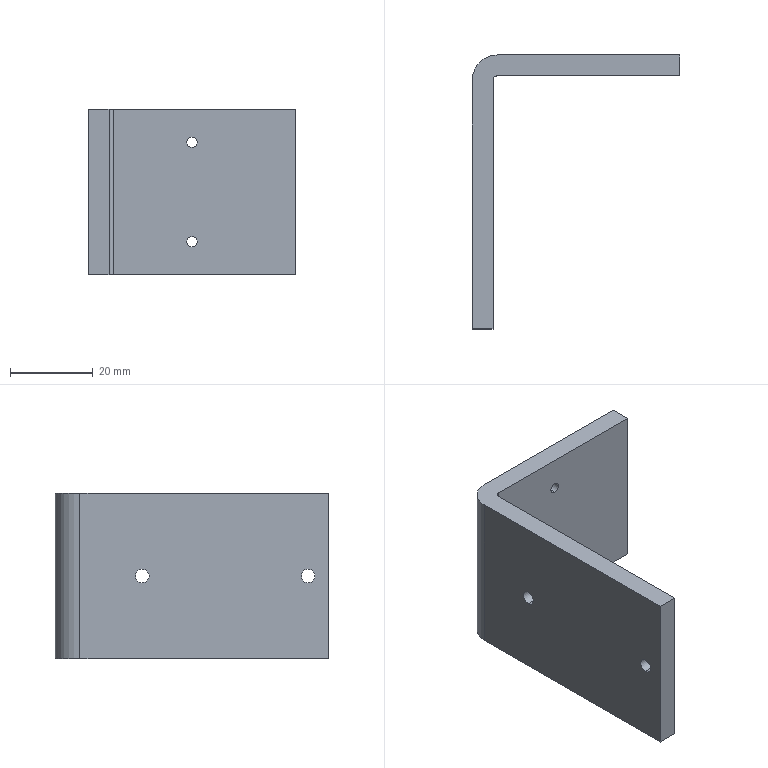Part | STEP file | X77-04302 | 1 solid | 18 faces | box 50 x 66 x 40 mm | volume 21765 mm3 | cylinder 10 | plane 8 | commonest cylinder face diameters 2.5 x4 3.3 x4 2 x1 12 x1
STEP:
#1=CARTESIAN_POINT('',(-24.91,-36.8,13.25));
#2=VERTEX_POINT('',#1);
#3=CARTESIAN_POINT('',(-24.91,-36.8,10.75));
#4=VERTEX_POINT('',#3);
#5=CARTESIAN_POINT('',(-24.91,-36.8,12.));
#6=DIRECTION('',(0.,-1.,0.));
#7=DIRECTION('',(1.,0.,0.));
#8=AXIS2_PLACEMENT_3D('',#5,#6,#7);
#9=CIRCLE('',#8,1.25);
#10=EDGE_CURVE('',#2,#4,#9,.T.);
#11=ORIENTED_EDGE('',*,*,#10,.T.);
#12=CARTESIAN_POINT('',(-24.91,-31.8,10.75));
#13=VERTEX_POINT('',#12);
#14=CARTESIAN_POINT('',(-24.91,-31.8,10.75));
#15=DIRECTION('',(0.,1.,0.));
#16=VECTOR('',#15,1000.);
#17=LINE('',#14,#16);
#18=EDGE_CURVE('',#4,#13,#17,.T.);
#19=ORIENTED_EDGE('',*,*,#18,.T.);
#20=CARTESIAN_POINT('',(-24.91,-31.8,13.25));
#21=VERTEX_POINT('',#20);
#22=CARTESIAN_POINT('',(-24.91,-31.8,12.));
#23=DIRECTION('',(0.,1.,0.));
#24=DIRECTION('',(0.,0.,1.));
#25=AXIS2_PLACEMENT_3D('',#22,#23,#24);
#26=CIRCLE('',#25,1.25);
#27=EDGE_CURVE('',#13,#21,#26,.T.);
#28=ORIENTED_EDGE('',*,*,#27,.T.);
#29=CARTESIAN_POINT('',(-24.91,-31.8,13.25));
#30=DIRECTION('',(0.,1.,0.));
#31=VECTOR('',#30,1000.);
#32=LINE('',#29,#31);
#33=EDGE_CURVE('',#2,#21,#32,.T.);
#34=ORIENTED_EDGE('',*,*,#33,.F.);
#35=EDGE_LOOP('',(#11,#19,#28,#34));
#36=FACE_OUTER_BOUND('',#35,.T.);
#37=CARTESIAN_POINT('',(-24.91,-31.8,12.));
#38=DIRECTION('',(0.,1.,0.));
#39=DIRECTION('',(0.,0.,1.));
#40=AXIS2_PLACEMENT_3D('',#37,#38,#39);
#41=CYLINDRICAL_SURFACE('',#40,1.25);
#42=ADVANCED_FACE('',(#36),#41,.F.);
#43=CARTESIAN_POINT('',(-24.91,-36.8,-10.75));
#44=VERTEX_POINT('',#43);
#45=CARTESIAN_POINT('',(-24.91,-36.8,-13.25));
#46=VERTEX_POINT('',#45);
#47=CARTESIAN_POINT('',(-24.91,-36.8,-12.));
#48=DIRECTION('',(0.,-1.,0.));
#49=DIRECTION('',(1.,0.,0.));
#50=AXIS2_PLACEMENT_3D('',#47,#48,#49);
#51=CIRCLE('',#50,1.25);
#52=EDGE_CURVE('',#44,#46,#51,.T.);
#53=ORIENTED_EDGE('',*,*,#52,.T.);
#54=CARTESIAN_POINT('',(-24.91,-31.8,-13.25));
#55=VERTEX_POINT('',#54);
#56=CARTESIAN_POINT('',(-24.91,-31.8,-13.25));
#57=DIRECTION('',(0.,1.,0.));
#58=VECTOR('',#57,1000.);
#59=LINE('',#56,#58);
#60=EDGE_CURVE('',#46,#55,#59,.T.);
#61=ORIENTED_EDGE('',*,*,#60,.T.);
#62=CARTESIAN_POINT('',(-24.91,-31.8,-10.75));
#63=VERTEX_POINT('',#62);
#64=CARTESIAN_POINT('',(-24.91,-31.8,-12.));
#65=DIRECTION('',(0.,1.,0.));
#66=DIRECTION('',(0.,0.,1.));
#67=AXIS2_PLACEMENT_3D('',#64,#65,#66);
#68=CIRCLE('',#67,1.25);
#69=EDGE_CURVE('',#55,#63,#68,.T.);
#70=ORIENTED_EDGE('',*,*,#69,.T.);
#71=CARTESIAN_POINT('',(-24.91,-31.8,-10.75));
#72=DIRECTION('',(0.,1.,0.));
#73=VECTOR('',#72,1000.);
#74=LINE('',#71,#73);
#75=EDGE_CURVE('',#44,#63,#74,.T.);
#76=ORIENTED_EDGE('',*,*,#75,.F.);
#77=EDGE_LOOP('',(#53,#61,#70,#76));
#78=FACE_OUTER_BOUND('',#77,.T.);
#79=CARTESIAN_POINT('',(-24.91,-31.8,-12.));
#80=DIRECTION('',(0.,1.,0.));
#81=DIRECTION('',(0.,0.,1.));
#82=AXIS2_PLACEMENT_3D('',#79,#80,#81);
#83=CYLINDRICAL_SURFACE('',#82,1.25);
#84=ADVANCED_FACE('',(#78),#83,.F.);
#85=CARTESIAN_POINT('',(-44.91,-92.8,1.65));
#86=VERTEX_POINT('',#85);
#87=CARTESIAN_POINT('',(-44.91,-92.8,-1.65));
#88=VERTEX_POINT('',#87);
#89=CARTESIAN_POINT('',(-44.91,-92.8,0.));
#90=DIRECTION('',(1.,0.,0.));
#91=DIRECTION('',(0.,0.,-1.));
#92=AXIS2_PLACEMENT_3D('',#89,#90,#91);
#93=CIRCLE('',#92,1.65);
#94=EDGE_CURVE('',#86,#88,#93,.T.);
#95=ORIENTED_EDGE('',*,*,#94,.T.);
#96=CARTESIAN_POINT('',(-49.91,-92.8,-1.65));
#97=VERTEX_POINT('',#96);
#98=CARTESIAN_POINT('',(-49.91,-92.8,-1.65));
#99=DIRECTION('',(-1.,0.,0.));
#100=VECTOR('',#99,1000.);
#101=LINE('',#98,#100);
#102=EDGE_CURVE('',#88,#97,#101,.T.);
#103=ORIENTED_EDGE('',*,*,#102,.T.);
#104=CARTESIAN_POINT('',(-49.91,-92.8,1.65));
#105=VERTEX_POINT('',#104);
#106=CARTESIAN_POINT('',(-49.91,-92.8,0.));
#107=DIRECTION('',(-1.,0.,0.));
#108=DIRECTION('',(0.,0.,1.));
#109=AXIS2_PLACEMENT_3D('',#106,#107,#108);
#110=CIRCLE('',#109,1.65);
#111=EDGE_CURVE('',#97,#105,#110,.T.);
#112=ORIENTED_EDGE('',*,*,#111,.T.);
#113=CARTESIAN_POINT('',(-49.91,-92.8,1.65));
#114=DIRECTION('',(-1.,0.,0.));
#115=VECTOR('',#114,1000.);
#116=LINE('',#113,#115);
#117=EDGE_CURVE('',#86,#105,#116,.T.);
#118=ORIENTED_EDGE('',*,*,#117,.F.);
#119=EDGE_LOOP('',(#95,#103,#112,#118));
#120=FACE_OUTER_BOUND('',#119,.T.);
#121=CARTESIAN_POINT('',(-49.91,-92.8,0.));
#122=DIRECTION('',(-1.,0.,0.));
#123=DIRECTION('',(0.,0.,1.));
#124=AXIS2_PLACEMENT_3D('',#121,#122,#123);
#125=CYLINDRICAL_SURFACE('',#124,1.65);
#126=ADVANCED_FACE('',(#120),#125,.F.);
#127=CARTESIAN_POINT('',(-44.91,-52.8,1.65));
#128=VERTEX_POINT('',#127);
#129=CARTESIAN_POINT('',(-44.91,-52.8,-1.65));
#130=VERTEX_POINT('',#129);
#131=CARTESIAN_POINT('',(-44.91,-52.8,0.));
#132=DIRECTION('',(1.,0.,0.));
#133=DIRECTION('',(0.,0.,-1.));
#134=AXIS2_PLACEMENT_3D('',#131,#132,#133);
#135=CIRCLE('',#134,1.65);
#136=EDGE_CURVE('',#128,#130,#135,.T.);
#137=ORIENTED_EDGE('',*,*,#136,.T.);
#138=CARTESIAN_POINT('',(-49.91,-52.8,-1.65));
#139=VERTEX_POINT('',#138);
#140=CARTESIAN_POINT('',(-49.91,-52.8,-1.65));
#141=DIRECTION('',(-1.,0.,0.));
#142=VECTOR('',#141,1000.);
#143=LINE('',#140,#142);
#144=EDGE_CURVE('',#130,#139,#143,.T.);
#145=ORIENTED_EDGE('',*,*,#144,.T.);
#146=CARTESIAN_POINT('',(-49.91,-52.8,1.65));
#147=VERTEX_POINT('',#146);
#148=CARTESIAN_POINT('',(-49.91,-52.8,0.));
#149=DIRECTION('',(-1.,0.,0.));
#150=DIRECTION('',(0.,0.,1.));
#151=AXIS2_PLACEMENT_3D('',#148,#149,#150);
#152=CIRCLE('',#151,1.65);
#153=EDGE_CURVE('',#139,#147,#152,.T.);
#154=ORIENTED_EDGE('',*,*,#153,.T.);
#155=CARTESIAN_POINT('',(-49.91,-52.8,1.65));
#156=DIRECTION('',(-1.,0.,0.));
#157=VECTOR('',#156,1000.);
#158=LINE('',#155,#157);
#159=EDGE_CURVE('',#128,#147,#158,.T.);
#160=ORIENTED_EDGE('',*,*,#159,.F.);
#161=EDGE_LOOP('',(#137,#145,#154,#160));
#162=FACE_OUTER_BOUND('',#161,.T.);
#163=CARTESIAN_POINT('',(-49.91,-52.8,0.));
#164=DIRECTION('',(-1.,0.,0.));
#165=DIRECTION('',(0.,0.,1.));
#166=AXIS2_PLACEMENT_3D('',#163,#164,#165);
#167=CYLINDRICAL_SURFACE('',#166,1.65);
#168=ADVANCED_FACE('',(#162),#167,.F.);
#169=CARTESIAN_POINT('',(0.09,-31.8,-20.));
#170=VERTEX_POINT('',#169);
#171=CARTESIAN_POINT('',(0.09,-31.8,20.));
#172=VERTEX_POINT('',#171);
#173=CARTESIAN_POINT('',(0.09,-31.8,-20.));
#174=DIRECTION('',(0.,0.,1.));
#175=VECTOR('',#174,1000.);
#176=LINE('',#173,#175);
#177=EDGE_CURVE('',#170,#172,#176,.T.);
#178=ORIENTED_EDGE('',*,*,#177,.T.);
#179=CARTESIAN_POINT('',(0.09,-36.8,20.));
#180=VERTEX_POINT('',#179);
#181=CARTESIAN_POINT('',(0.09,-31.8,20.));
#182=DIRECTION('',(0.,1.,0.));
#183=VECTOR('',#182,1000.);
#184=LINE('',#181,#183);
#185=EDGE_CURVE('',#180,#172,#184,.T.);
#186=ORIENTED_EDGE('',*,*,#185,.F.);
#187=CARTESIAN_POINT('',(0.09,-36.8,-20.));
#188=VERTEX_POINT('',#187);
#189=CARTESIAN_POINT('',(0.09,-36.8,-20.));
#190=DIRECTION('',(0.,0.,1.));
#191=VECTOR('',#190,1000.);
#192=LINE('',#189,#191);
#193=EDGE_CURVE('',#188,#180,#192,.T.);
#194=ORIENTED_EDGE('',*,*,#193,.F.);
#195=CARTESIAN_POINT('',(0.09,-31.8,-20.));
#196=DIRECTION('',(0.,1.,0.));
#197=VECTOR('',#196,1000.);
#198=LINE('',#195,#197);
#199=EDGE_CURVE('',#188,#170,#198,.T.);
#200=ORIENTED_EDGE('',*,*,#199,.T.);
#201=EDGE_LOOP('',(#178,#186,#194,#200));
#202=FACE_OUTER_BOUND('',#201,.T.);
#203=CARTESIAN_POINT('',(0.09,-31.8,-20.));
#204=DIRECTION('',(1.,0.,0.));
#205=DIRECTION('',(0.,1.,0.));
#206=AXIS2_PLACEMENT_3D('',#203,#204,#205);
#207=PLANE('',#206);
#208=ADVANCED_FACE('',(#202),#207,.T.);
#209=ORIENTED_EDGE('',*,*,#10,.F.);
#210=CARTESIAN_POINT('',(-24.91,-36.8,12.));
#211=DIRECTION('',(0.,-1.,0.));
#212=DIRECTION('',(1.,0.,0.));
#213=AXIS2_PLACEMENT_3D('',#210,#211,#212);
#214=CIRCLE('',#213,1.25);
#215=EDGE_CURVE('',#4,#2,#214,.T.);
#216=ORIENTED_EDGE('',*,*,#215,.F.);
#217=EDGE_LOOP('',(#209,#216));
#218=FACE_BOUND('',#217,.T.);
#219=ORIENTED_EDGE('',*,*,#52,.F.);
#220=CARTESIAN_POINT('',(-24.91,-36.8,-12.));
#221=DIRECTION('',(0.,-1.,0.));
#222=DIRECTION('',(1.,0.,0.));
#223=AXIS2_PLACEMENT_3D('',#220,#221,#222);
#224=CIRCLE('',#223,1.25);
#225=EDGE_CURVE('',#46,#44,#224,.T.);
#226=ORIENTED_EDGE('',*,*,#225,.F.);
#227=EDGE_LOOP('',(#219,#226));
#228=FACE_BOUND('',#227,.T.);
#229=ORIENTED_EDGE('',*,*,#193,.T.);
#230=CARTESIAN_POINT('',(-43.91,-36.8,20.));
#231=VERTEX_POINT('',#230);
#232=CARTESIAN_POINT('',(0.09,-36.8,20.));
#233=DIRECTION('',(1.,0.,0.));
#234=VECTOR('',#233,1000.);
#235=LINE('',#232,#234);
#236=EDGE_CURVE('',#231,#180,#235,.T.);
#237=ORIENTED_EDGE('',*,*,#236,.F.);
#238=CARTESIAN_POINT('',(-43.91,-36.8,-20.));
#239=VERTEX_POINT('',#238);
#240=CARTESIAN_POINT('',(-43.91,-36.8,-20.));
#241=DIRECTION('',(0.,0.,1.));
#242=VECTOR('',#241,1000.);
#243=LINE('',#240,#242);
#244=EDGE_CURVE('',#239,#231,#243,.T.);
#245=ORIENTED_EDGE('',*,*,#244,.F.);
#246=CARTESIAN_POINT('',(0.09,-36.8,-20.));
#247=DIRECTION('',(1.,0.,0.));
#248=VECTOR('',#247,1000.);
#249=LINE('',#246,#248);
#250=EDGE_CURVE('',#239,#188,#249,.T.);
#251=ORIENTED_EDGE('',*,*,#250,.T.);
#252=EDGE_LOOP('',(#229,#237,#245,#251));
#253=FACE_OUTER_BOUND('',#252,.T.);
#254=CARTESIAN_POINT('',(0.09,-36.8,-20.));
#255=DIRECTION('',(0.,-1.,0.));
#256=DIRECTION('',(1.,0.,0.));
#257=AXIS2_PLACEMENT_3D('',#254,#255,#256);
#258=PLANE('',#257);
#259=ADVANCED_FACE('',(#218,#228,#253),#258,.T.);
#260=ORIENTED_EDGE('',*,*,#244,.T.);
#261=CARTESIAN_POINT('',(-44.91,-37.8,20.));
#262=VERTEX_POINT('',#261);
#263=CARTESIAN_POINT('',(-43.91,-37.8,20.));
#264=DIRECTION('',(0.,0.,-1.));
#265=DIRECTION('',(-1.,0.,0.));
#266=AXIS2_PLACEMENT_3D('',#263,#264,#265);
#267=CIRCLE('',#266,1.);
#268=EDGE_CURVE('',#262,#231,#267,.T.);
#269=ORIENTED_EDGE('',*,*,#268,.F.);
#270=CARTESIAN_POINT('',(-44.91,-37.8,-20.));
#271=VERTEX_POINT('',#270);
#272=CARTESIAN_POINT('',(-44.91,-37.8,-20.));
#273=DIRECTION('',(0.,0.,1.));
#274=VECTOR('',#273,1000.);
#275=LINE('',#272,#274);
#276=EDGE_CURVE('',#271,#262,#275,.T.);
#277=ORIENTED_EDGE('',*,*,#276,.F.);
#278=CARTESIAN_POINT('',(-43.91,-37.8,-20.));
#279=DIRECTION('',(0.,0.,-1.));
#280=DIRECTION('',(-1.,0.,0.));
#281=AXIS2_PLACEMENT_3D('',#278,#279,#280);
#282=CIRCLE('',#281,1.);
#283=EDGE_CURVE('',#271,#239,#282,.T.);
#284=ORIENTED_EDGE('',*,*,#283,.T.);
#285=EDGE_LOOP('',(#260,#269,#277,#284));
#286=FACE_OUTER_BOUND('',#285,.T.);
#287=CARTESIAN_POINT('',(-43.91,-37.8,-20.));
#288=DIRECTION('',(0.,0.,1.));
#289=DIRECTION('',(1.,0.,0.));
#290=AXIS2_PLACEMENT_3D('',#287,#288,#289);
#291=CYLINDRICAL_SURFACE('',#290,1.);
#292=ADVANCED_FACE('',(#286),#291,.F.);
#293=ORIENTED_EDGE('',*,*,#94,.F.);
#294=CARTESIAN_POINT('',(-44.91,-92.8,0.));
#295=DIRECTION('',(1.,0.,0.));
#296=DIRECTION('',(0.,0.,-1.));
#297=AXIS2_PLACEMENT_3D('',#294,#295,#296);
#298=CIRCLE('',#297,1.65);
#299=EDGE_CURVE('',#88,#86,#298,.T.);
#300=ORIENTED_EDGE('',*,*,#299,.F.);
#301=EDGE_LOOP('',(#293,#300));
#302=FACE_BOUND('',#301,.T.);
#303=ORIENTED_EDGE('',*,*,#136,.F.);
#304=CARTESIAN_POINT('',(-44.91,-52.8,0.));
#305=DIRECTION('',(1.,0.,0.));
#306=DIRECTION('',(0.,0.,-1.));
#307=AXIS2_PLACEMENT_3D('',#304,#305,#306);
#308=CIRCLE('',#307,1.65);
#309=EDGE_CURVE('',#130,#128,#308,.T.);
#310=ORIENTED_EDGE('',*,*,#309,.F.);
#311=EDGE_LOOP('',(#303,#310));
#312=FACE_BOUND('',#311,.T.);
#313=ORIENTED_EDGE('',*,*,#276,.T.);
#314=CARTESIAN_POINT('',(-44.91,-97.8,20.));
#315=VERTEX_POINT('',#314);
#316=CARTESIAN_POINT('',(-44.91,-37.8,20.));
#317=DIRECTION('',(0.,1.,0.));
#318=VECTOR('',#317,1000.);
#319=LINE('',#316,#318);
#320=EDGE_CURVE('',#315,#262,#319,.T.);
#321=ORIENTED_EDGE('',*,*,#320,.F.);
#322=CARTESIAN_POINT('',(-44.91,-97.8,-20.));
#323=VERTEX_POINT('',#322);
#324=CARTESIAN_POINT('',(-44.91,-97.8,-20.));
#325=DIRECTION('',(0.,0.,1.));
#326=VECTOR('',#325,1000.);
#327=LINE('',#324,#326);
#328=EDGE_CURVE('',#323,#315,#327,.T.);
#329=ORIENTED_EDGE('',*,*,#328,.F.);
#330=CARTESIAN_POINT('',(-44.91,-37.8,-20.));
#331=DIRECTION('',(0.,1.,0.));
#332=VECTOR('',#331,1000.);
#333=LINE('',#330,#332);
#334=EDGE_CURVE('',#323,#271,#333,.T.);
#335=ORIENTED_EDGE('',*,*,#334,.T.);
#336=EDGE_LOOP('',(#313,#321,#329,#335));
#337=FACE_OUTER_BOUND('',#336,.T.);
#338=CARTESIAN_POINT('',(-44.91,-37.8,-20.));
#339=DIRECTION('',(1.,0.,0.));
#340=DIRECTION('',(0.,0.,-1.));
#341=AXIS2_PLACEMENT_3D('',#338,#339,#340);
#342=PLANE('',#341);
#343=ADVANCED_FACE('',(#302,#312,#337),#342,.T.);
#344=ORIENTED_EDGE('',*,*,#328,.T.);
#345=CARTESIAN_POINT('',(-49.91,-97.8,20.));
#346=VERTEX_POINT('',#345);
#347=CARTESIAN_POINT('',(-49.91,-97.8,20.));
#348=DIRECTION('',(1.,0.,0.));
#349=VECTOR('',#348,1000.);
#350=LINE('',#347,#349);
#351=EDGE_CURVE('',#346,#315,#350,.T.);
#352=ORIENTED_EDGE('',*,*,#351,.F.);
#353=CARTESIAN_POINT('',(-49.91,-97.8,-20.));
#354=VERTEX_POINT('',#353);
#355=CARTESIAN_POINT('',(-49.91,-97.8,-20.));
#356=DIRECTION('',(0.,0.,1.));
#357=VECTOR('',#356,1000.);
#358=LINE('',#355,#357);
#359=EDGE_CURVE('',#354,#346,#358,.T.);
#360=ORIENTED_EDGE('',*,*,#359,.F.);
#361=CARTESIAN_POINT('',(-49.91,-97.8,-20.));
#362=DIRECTION('',(1.,0.,0.));
#363=VECTOR('',#362,1000.);
#364=LINE('',#361,#363);
#365=EDGE_CURVE('',#354,#323,#364,.T.);
#366=ORIENTED_EDGE('',*,*,#365,.T.);
#367=EDGE_LOOP('',(#344,#352,#360,#366));
#368=FACE_OUTER_BOUND('',#367,.T.);
#369=CARTESIAN_POINT('',(-49.91,-97.8,-20.));
#370=DIRECTION('',(0.,-1.,0.));
#371=DIRECTION('',(1.,0.,0.));
#372=AXIS2_PLACEMENT_3D('',#369,#370,#371);
#373=PLANE('',#372);
#374=ADVANCED_FACE('',(#368),#373,.T.);
#375=CARTESIAN_POINT('',(-49.91,-92.8,0.));
#376=DIRECTION('',(-1.,0.,0.));
#377=DIRECTION('',(0.,0.,1.));
#378=AXIS2_PLACEMENT_3D('',#375,#376,#377);
#379=CIRCLE('',#378,1.65);
#380=EDGE_CURVE('',#105,#97,#379,.T.);
#381=ORIENTED_EDGE('',*,*,#380,.F.);
#382=ORIENTED_EDGE('',*,*,#111,.F.);
#383=EDGE_LOOP('',(#381,#382));
#384=FACE_BOUND('',#383,.T.);
#385=CARTESIAN_POINT('',(-49.91,-52.8,0.));
#386=DIRECTION('',(-1.,0.,0.));
#387=DIRECTION('',(0.,0.,1.));
#388=AXIS2_PLACEMENT_3D('',#385,#386,#387);
#389=CIRCLE('',#388,1.65);
#390=EDGE_CURVE('',#147,#139,#389,.T.);
#391=ORIENTED_EDGE('',*,*,#390,.F.);
#392=ORIENTED_EDGE('',*,*,#153,.F.);
#393=EDGE_LOOP('',(#391,#392));
#394=FACE_BOUND('',#393,.T.);
#395=ORIENTED_EDGE('',*,*,#359,.T.);
#396=CARTESIAN_POINT('',(-49.91,-37.8,20.));
#397=VERTEX_POINT('',#396);
#398=CARTESIAN_POINT('',(-49.91,-37.8,20.));
#399=DIRECTION('',(0.,-1.,0.));
#400=VECTOR('',#399,1000.);
#401=LINE('',#398,#400);
#402=EDGE_CURVE('',#397,#346,#401,.T.);
#403=ORIENTED_EDGE('',*,*,#402,.F.);
#404=CARTESIAN_POINT('',(-49.91,-37.8,-20.));
#405=VERTEX_POINT('',#404);
#406=CARTESIAN_POINT('',(-49.91,-37.8,-20.));
#407=DIRECTION('',(0.,0.,1.));
#408=VECTOR('',#407,1000.);
#409=LINE('',#406,#408);
#410=EDGE_CURVE('',#405,#397,#409,.T.);
#411=ORIENTED_EDGE('',*,*,#410,.F.);
#412=CARTESIAN_POINT('',(-49.91,-37.8,-20.));
#413=DIRECTION('',(0.,-1.,0.));
#414=VECTOR('',#413,1000.);
#415=LINE('',#412,#414);
#416=EDGE_CURVE('',#405,#354,#415,.T.);
#417=ORIENTED_EDGE('',*,*,#416,.T.);
#418=EDGE_LOOP('',(#395,#403,#411,#417));
#419=FACE_OUTER_BOUND('',#418,.T.);
#420=CARTESIAN_POINT('',(-49.91,-37.8,-20.));
#421=DIRECTION('',(-1.,0.,0.));
#422=DIRECTION('',(0.,-1.,0.));
#423=AXIS2_PLACEMENT_3D('',#420,#421,#422);
#424=PLANE('',#423);
#425=ADVANCED_FACE('',(#384,#394,#419),#424,.T.);
#426=ORIENTED_EDGE('',*,*,#410,.T.);
#427=CARTESIAN_POINT('',(-43.91,-31.8,20.));
#428=VERTEX_POINT('',#427);
#429=CARTESIAN_POINT('',(-43.91,-37.8,20.));
#430=DIRECTION('',(0.,0.,1.));
#431=DIRECTION('',(-1.,0.,0.));
#432=AXIS2_PLACEMENT_3D('',#429,#430,#431);
#433=CIRCLE('',#432,6.);
#434=EDGE_CURVE('',#428,#397,#433,.T.);
#435=ORIENTED_EDGE('',*,*,#434,.F.);
#436=CARTESIAN_POINT('',(-43.91,-31.8,-20.));
#437=VERTEX_POINT('',#436);
#438=CARTESIAN_POINT('',(-43.91,-31.8,-20.));
#439=DIRECTION('',(0.,0.,1.));
#440=VECTOR('',#439,1000.);
#441=LINE('',#438,#440);
#442=EDGE_CURVE('',#437,#428,#441,.T.);
#443=ORIENTED_EDGE('',*,*,#442,.F.);
#444=CARTESIAN_POINT('',(-43.91,-37.8,-20.));
#445=DIRECTION('',(0.,0.,1.));
#446=DIRECTION('',(-1.,0.,0.));
#447=AXIS2_PLACEMENT_3D('',#444,#445,#446);
#448=CIRCLE('',#447,6.);
#449=EDGE_CURVE('',#437,#405,#448,.T.);
#450=ORIENTED_EDGE('',*,*,#449,.T.);
#451=EDGE_LOOP('',(#426,#435,#443,#450));
#452=FACE_OUTER_BOUND('',#451,.T.);
#453=CARTESIAN_POINT('',(-43.91,-37.8,-20.));
#454=DIRECTION('',(0.,0.,1.));
#455=DIRECTION('',(1.,0.,0.));
#456=AXIS2_PLACEMENT_3D('',#453,#454,#455);
#457=CYLINDRICAL_SURFACE('',#456,6.);
#458=ADVANCED_FACE('',(#452),#457,.T.);
#459=CARTESIAN_POINT('',(-24.91,-31.8,12.));
#460=DIRECTION('',(0.,1.,0.));
#461=DIRECTION('',(0.,0.,1.));
#462=AXIS2_PLACEMENT_3D('',#459,#460,#461);
#463=CIRCLE('',#462,1.25);
#464=EDGE_CURVE('',#21,#13,#463,.T.);
#465=ORIENTED_EDGE('',*,*,#464,.F.);
#466=ORIENTED_EDGE('',*,*,#27,.F.);
#467=EDGE_LOOP('',(#465,#466));
#468=FACE_BOUND('',#467,.T.);
#469=CARTESIAN_POINT('',(-24.91,-31.8,-12.));
#470=DIRECTION('',(0.,1.,0.));
#471=DIRECTION('',(0.,0.,1.));
#472=AXIS2_PLACEMENT_3D('',#469,#470,#471);
#473=CIRCLE('',#472,1.25);
#474=EDGE_CURVE('',#63,#55,#473,.T.);
#475=ORIENTED_EDGE('',*,*,#474,.F.);
#476=ORIENTED_EDGE('',*,*,#69,.F.);
#477=EDGE_LOOP('',(#475,#476));
#478=FACE_BOUND('',#477,.T.);
#479=ORIENTED_EDGE('',*,*,#442,.T.);
#480=CARTESIAN_POINT('',(0.09,-31.8,20.));
#481=DIRECTION('',(-1.,0.,0.));
#482=VECTOR('',#481,1000.);
#483=LINE('',#480,#482);
#484=EDGE_CURVE('',#172,#428,#483,.T.);
#485=ORIENTED_EDGE('',*,*,#484,.F.);
#486=ORIENTED_EDGE('',*,*,#177,.F.);
#487=CARTESIAN_POINT('',(0.09,-31.8,-20.));
#488=DIRECTION('',(-1.,0.,0.));
#489=VECTOR('',#488,1000.);
#490=LINE('',#487,#489);
#491=EDGE_CURVE('',#170,#437,#490,.T.);
#492=ORIENTED_EDGE('',*,*,#491,.T.);
#493=EDGE_LOOP('',(#479,#485,#486,#492));
#494=FACE_OUTER_BOUND('',#493,.T.);
#495=CARTESIAN_POINT('',(0.09,-31.8,-20.));
#496=DIRECTION('',(0.,1.,0.));
#497=DIRECTION('',(-1.,0.,0.));
#498=AXIS2_PLACEMENT_3D('',#495,#496,#497);
#499=PLANE('',#498);
#500=ADVANCED_FACE('',(#468,#478,#494),#499,.T.);
#501=ORIENTED_EDGE('',*,*,#199,.F.);
#502=ORIENTED_EDGE('',*,*,#250,.F.);
#503=ORIENTED_EDGE('',*,*,#283,.F.);
#504=ORIENTED_EDGE('',*,*,#334,.F.);
#505=ORIENTED_EDGE('',*,*,#365,.F.);
#506=ORIENTED_EDGE('',*,*,#416,.F.);
#507=ORIENTED_EDGE('',*,*,#449,.F.);
#508=ORIENTED_EDGE('',*,*,#491,.F.);
#509=EDGE_LOOP('',(#501,#502,#503,#504,#505,#506,#507,#508));
#510=FACE_OUTER_BOUND('',#509,.T.);
#511=CARTESIAN_POINT('',(-43.91,-37.8,-20.));
#512=DIRECTION('',(0.,0.,-1.));
#513=DIRECTION('',(-1.,0.,0.));
#514=AXIS2_PLACEMENT_3D('',#511,#512,#513);
#515=PLANE('',#514);
#516=ADVANCED_FACE('',(#510),#515,.T.);
#517=ORIENTED_EDGE('',*,*,#185,.T.);
#518=ORIENTED_EDGE('',*,*,#484,.T.);
#519=ORIENTED_EDGE('',*,*,#434,.T.);
#520=ORIENTED_EDGE('',*,*,#402,.T.);
#521=ORIENTED_EDGE('',*,*,#351,.T.);
#522=ORIENTED_EDGE('',*,*,#320,.T.);
#523=ORIENTED_EDGE('',*,*,#268,.T.);
#524=ORIENTED_EDGE('',*,*,#236,.T.);
#525=EDGE_LOOP('',(#517,#518,#519,#520,#521,#522,#523,#524));
#526=FACE_OUTER_BOUND('',#525,.T.);
#527=CARTESIAN_POINT('',(-43.91,-37.8,20.));
#528=DIRECTION('',(0.,0.,-1.));
#529=DIRECTION('',(-1.,0.,0.));
#530=AXIS2_PLACEMENT_3D('',#527,#528,#529);
#531=PLANE('',#530);
#532=ADVANCED_FACE('',(#526),#531,.F.);
#533=ORIENTED_EDGE('',*,*,#144,.F.);
#534=ORIENTED_EDGE('',*,*,#309,.T.);
#535=ORIENTED_EDGE('',*,*,#159,.T.);
#536=ORIENTED_EDGE('',*,*,#390,.T.);
#537=EDGE_LOOP('',(#533,#534,#535,#536));
#538=FACE_OUTER_BOUND('',#537,.T.);
#539=CARTESIAN_POINT('',(-49.91,-52.8,0.));
#540=DIRECTION('',(-1.,0.,0.));
#541=DIRECTION('',(0.,0.,1.));
#542=AXIS2_PLACEMENT_3D('',#539,#540,#541);
#543=CYLINDRICAL_SURFACE('',#542,1.65);
#544=ADVANCED_FACE('',(#538),#543,.F.);
#545=ORIENTED_EDGE('',*,*,#102,.F.);
#546=ORIENTED_EDGE('',*,*,#299,.T.);
#547=ORIENTED_EDGE('',*,*,#117,.T.);
#548=ORIENTED_EDGE('',*,*,#380,.T.);
#549=EDGE_LOOP('',(#545,#546,#547,#548));
#550=FACE_OUTER_BOUND('',#549,.T.);
#551=CARTESIAN_POINT('',(-49.91,-92.8,0.));
#552=DIRECTION('',(-1.,0.,0.));
#553=DIRECTION('',(0.,0.,1.));
#554=AXIS2_PLACEMENT_3D('',#551,#552,#553);
#555=CYLINDRICAL_SURFACE('',#554,1.65);
#556=ADVANCED_FACE('',(#550),#555,.F.);
#557=ORIENTED_EDGE('',*,*,#60,.F.);
#558=ORIENTED_EDGE('',*,*,#225,.T.);
#559=ORIENTED_EDGE('',*,*,#75,.T.);
#560=ORIENTED_EDGE('',*,*,#474,.T.);
#561=EDGE_LOOP('',(#557,#558,#559,#560));
#562=FACE_OUTER_BOUND('',#561,.T.);
#563=CARTESIAN_POINT('',(-24.91,-31.8,-12.));
#564=DIRECTION('',(0.,1.,0.));
#565=DIRECTION('',(0.,0.,1.));
#566=AXIS2_PLACEMENT_3D('',#563,#564,#565);
#567=CYLINDRICAL_SURFACE('',#566,1.25);
#568=ADVANCED_FACE('',(#562),#567,.F.);
#569=ORIENTED_EDGE('',*,*,#18,.F.);
#570=ORIENTED_EDGE('',*,*,#215,.T.);
#571=ORIENTED_EDGE('',*,*,#33,.T.);
#572=ORIENTED_EDGE('',*,*,#464,.T.);
#573=EDGE_LOOP('',(#569,#570,#571,#572));
#574=FACE_OUTER_BOUND('',#573,.T.);
#575=CARTESIAN_POINT('',(-24.91,-31.8,12.));
#576=DIRECTION('',(0.,1.,0.));
#577=DIRECTION('',(0.,0.,1.));
#578=AXIS2_PLACEMENT_3D('',#575,#576,#577);
#579=CYLINDRICAL_SURFACE('',#578,1.25);
#580=ADVANCED_FACE('',(#574),#579,.F.);
#581=CLOSED_SHELL('',(#42,#84,#126,#168,#208,#259,#292,#343,#374,#425,#458,#500,#516,#532,#544,#556,#568,#580));
#582=MANIFOLD_SOLID_BREP('',#581);
#583=CARTESIAN_POINT('',(0.,0.,0.));
#584=DIRECTION('',(0.,0.,1.));
#585=DIRECTION('',(1.,0.,0.));
#586=AXIS2_PLACEMENT_3D('',#583,#584,#585);
#587=(LENGTH_UNIT()NAMED_UNIT(*)SI_UNIT(.MILLI.,.METRE.));
#588=UNCERTAINTY_MEASURE_WITH_UNIT(LENGTH_MEASURE(0.00001),#587,'','');
#589=(NAMED_UNIT(*)PLANE_ANGLE_UNIT()SI_UNIT($,.RADIAN.));
#590=(NAMED_UNIT(*)SI_UNIT($,.STERADIAN.)SOLID_ANGLE_UNIT());
#591=(GEOMETRIC_REPRESENTATION_CONTEXT(3)GLOBAL_UNCERTAINTY_ASSIGNED_CONTEXT((#588))GLOBAL_UNIT_ASSIGNED_CONTEXT((#587,#589,#590))REPRESENTATION_CONTEXT('',''));
#592=ADVANCED_BREP_SHAPE_REPRESENTATION('',(#582,#586),#591);